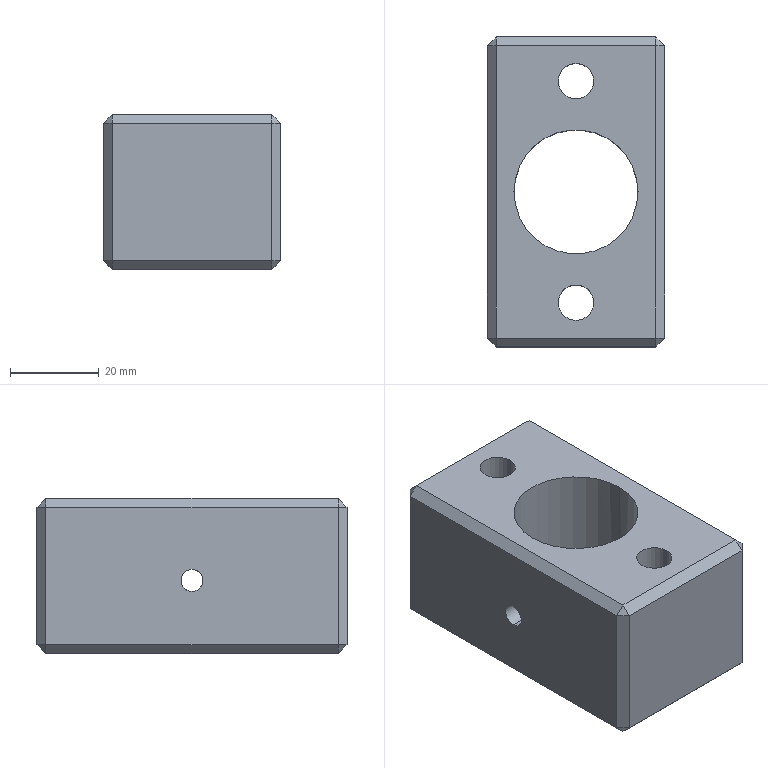Part | SolidWorks | features ICE 2, MirrorPattern 2, 3DProfileFeature 1, Chamfer 1, Extrusion 1, HoleWzd 1 | 1 solid | 36 faces | box 40 x 70 x 35 mm | volume 71575 mm3 | plane 26 | cylinder 10 | commonest cylinder face diameters 5 x4 8 x4 28 x2
STEP:
#1=CARTESIAN_POINT('',(14.,0.,13.999));
#2=VERTEX_POINT('',#1);
#3=CARTESIAN_POINT('',(14.,0.,18.999));
#4=VERTEX_POINT('',#3);
#5=CARTESIAN_POINT('',(14.,0.,13.999));
#6=CARTESIAN_POINT('',(14.,-0.1655,13.999));
#7=CARTESIAN_POINT('',(13.997,-0.3282,14.015));
#8=CARTESIAN_POINT('',(13.986,-0.6482,14.079));
#9=CARTESIAN_POINT('',(13.978,-0.8072,14.127));
#10=CARTESIAN_POINT('',(13.957,-1.11,14.253));
#11=CARTESIAN_POINT('',(13.944,-1.253,14.33));
#12=CARTESIAN_POINT('',(13.917,-1.525,14.511));
#13=CARTESIAN_POINT('',(13.903,-1.653,14.616));
#14=CARTESIAN_POINT('',(13.859,-1.998,14.962));
#15=CARTESIAN_POINT('',(13.829,-2.184,15.24));
#16=CARTESIAN_POINT('',(13.798,-2.372,15.691));
#17=CARTESIAN_POINT('',(13.789,-2.42,15.849));
#18=CARTESIAN_POINT('',(13.778,-2.484,16.172));
#19=CARTESIAN_POINT('',(13.775,-2.5,16.334));
#20=CARTESIAN_POINT('',(13.775,-2.5,16.661));
#21=CARTESIAN_POINT('',(13.778,-2.484,16.827));
#22=CARTESIAN_POINT('',(13.789,-2.42,17.148));
#23=CARTESIAN_POINT('',(13.798,-2.372,17.304));
#24=CARTESIAN_POINT('',(13.819,-2.247,17.607));
#25=CARTESIAN_POINT('',(13.831,-2.169,17.753));
#26=CARTESIAN_POINT('',(13.858,-1.988,18.024));
#27=CARTESIAN_POINT('',(13.873,-1.884,18.15));
#28=CARTESIAN_POINT('',(13.903,-1.651,18.383));
#29=CARTESIAN_POINT('',(13.917,-1.525,18.486));
#30=CARTESIAN_POINT('',(13.944,-1.255,18.667));
#31=CARTESIAN_POINT('',(13.957,-1.109,18.746));
#32=CARTESIAN_POINT('',(13.978,-0.8062,18.871));
#33=CARTESIAN_POINT('',(13.986,-0.6504,18.918));
#34=CARTESIAN_POINT('',(13.997,-0.3293,18.982));
#35=CARTESIAN_POINT('',(14.,-0.1633,18.999));
#36=CARTESIAN_POINT('',(14.,0.,18.999));
#37=B_SPLINE_CURVE_WITH_KNOTS('',3,(#5,#6,#7,#8,#9,#10,#11,#12,#13,#14,#15,#16,#17,#18,#19,#20,#21,#22,#23,#24,#25,#26,#27,#28,#29,#30,#31,#32,#33,#34,#35,#36),.UNSPECIFIED.,.F.,.F.,(4,2,2,2,2,2,2,2,2,2,2,2,2,2,2,4),(0.,0.0004895,0.000979,0.001468,0.001958,0.002937,0.003426,0.003916,0.004405,0.004895,0.005384,0.005874,0.006363,0.006853,0.007342,0.007832),.UNSPECIFIED.);
#38=EDGE_CURVE('',#2,#4,#37,.T.);
#39=ORIENTED_EDGE('',*,*,#38,.T.);
#40=CARTESIAN_POINT('',(20.,0.,18.999));
#41=VERTEX_POINT('',#40);
#42=CARTESIAN_POINT('',(20.,0.,18.999));
#43=DIRECTION('',(1.,0.,0.));
#44=VECTOR('',#43,1000.);
#45=LINE('',#42,#44);
#46=EDGE_CURVE('',#4,#41,#45,.T.);
#47=ORIENTED_EDGE('',*,*,#46,.T.);
#48=CARTESIAN_POINT('',(20.,0.,13.999));
#49=VERTEX_POINT('',#48);
#50=CARTESIAN_POINT('',(20.,0.,16.499));
#51=DIRECTION('',(1.,0.,0.));
#52=DIRECTION('',(0.,0.,-1.));
#53=AXIS2_PLACEMENT_3D('',#50,#51,#52);
#54=CIRCLE('',#53,2.5);
#55=EDGE_CURVE('',#41,#49,#54,.T.);
#56=ORIENTED_EDGE('',*,*,#55,.T.);
#57=CARTESIAN_POINT('',(20.,0.,13.999));
#58=DIRECTION('',(1.,0.,0.));
#59=VECTOR('',#58,1000.);
#60=LINE('',#57,#59);
#61=EDGE_CURVE('',#2,#49,#60,.T.);
#62=ORIENTED_EDGE('',*,*,#61,.F.);
#63=EDGE_LOOP('',(#39,#47,#56,#62));
#64=FACE_OUTER_BOUND('',#63,.T.);
#65=CARTESIAN_POINT('',(20.,0.,16.499));
#66=DIRECTION('',(1.,0.,0.));
#67=DIRECTION('',(0.,0.,-1.));
#68=AXIS2_PLACEMENT_3D('',#65,#66,#67);
#69=CYLINDRICAL_SURFACE('',#68,2.5);
#70=ADVANCED_FACE('',(#64),#69,.F.);
#71=CARTESIAN_POINT('',(-4.,-25.,0.));
#72=VERTEX_POINT('',#71);
#73=CARTESIAN_POINT('',(4.,-25.,0.));
#74=VERTEX_POINT('',#73);
#75=CARTESIAN_POINT('',(0.,-25.,0.));
#76=DIRECTION('',(0.,0.,1.));
#77=DIRECTION('',(-1.,0.,0.));
#78=AXIS2_PLACEMENT_3D('',#75,#76,#77);
#79=CIRCLE('',#78,4.);
#80=EDGE_CURVE('',#72,#74,#79,.T.);
#81=ORIENTED_EDGE('',*,*,#80,.F.);
#82=CARTESIAN_POINT('',(-4.,-25.,35.));
#83=VERTEX_POINT('',#82);
#84=CARTESIAN_POINT('',(-4.,-25.,-24.));
#85=DIRECTION('',(0.,0.,1.));
#86=VECTOR('',#85,1000.);
#87=LINE('',#84,#86);
#88=EDGE_CURVE('',#72,#83,#87,.T.);
#89=ORIENTED_EDGE('',*,*,#88,.T.);
#90=CARTESIAN_POINT('',(4.,-25.,35.));
#91=VERTEX_POINT('',#90);
#92=CARTESIAN_POINT('',(0.,-25.,35.));
#93=DIRECTION('',(0.,0.,-1.));
#94=DIRECTION('',(1.,0.,0.));
#95=AXIS2_PLACEMENT_3D('',#92,#93,#94);
#96=CIRCLE('',#95,4.);
#97=EDGE_CURVE('',#91,#83,#96,.T.);
#98=ORIENTED_EDGE('',*,*,#97,.F.);
#99=CARTESIAN_POINT('',(4.,-25.,-24.));
#100=DIRECTION('',(0.,0.,1.));
#101=VECTOR('',#100,1000.);
#102=LINE('',#99,#101);
#103=EDGE_CURVE('',#74,#91,#102,.T.);
#104=ORIENTED_EDGE('',*,*,#103,.F.);
#105=EDGE_LOOP('',(#81,#89,#98,#104));
#106=FACE_OUTER_BOUND('',#105,.T.);
#107=CARTESIAN_POINT('',(0.,-25.,-24.));
#108=DIRECTION('',(0.,0.,1.));
#109=DIRECTION('',(1.,0.,0.));
#110=AXIS2_PLACEMENT_3D('',#107,#108,#109);
#111=CYLINDRICAL_SURFACE('',#110,4.);
#112=ADVANCED_FACE('',(#106),#111,.F.);
#113=CARTESIAN_POINT('',(-14.,0.,13.999));
#114=VERTEX_POINT('',#113);
#115=CARTESIAN_POINT('',(-14.,0.,18.999));
#116=VERTEX_POINT('',#115);
#117=CARTESIAN_POINT('',(-14.,0.,13.999));
#118=CARTESIAN_POINT('',(-14.,-0.3266,13.999));
#119=CARTESIAN_POINT('',(-13.988,-0.6561,14.065));
#120=CARTESIAN_POINT('',(-13.957,-1.108,14.252));
#121=CARTESIAN_POINT('',(-13.944,-1.253,14.33));
#122=CARTESIAN_POINT('',(-13.917,-1.526,14.512));
#123=CARTESIAN_POINT('',(-13.903,-1.651,14.615));
#124=CARTESIAN_POINT('',(-13.873,-1.882,14.845));
#125=CARTESIAN_POINT('',(-13.859,-1.987,14.973));
#126=CARTESIAN_POINT('',(-13.831,-2.169,15.244));
#127=CARTESIAN_POINT('',(-13.819,-2.246,15.388));
#128=CARTESIAN_POINT('',(-13.798,-2.371,15.691));
#129=CARTESIAN_POINT('',(-13.789,-2.42,15.849));
#130=CARTESIAN_POINT('',(-13.778,-2.483,16.169));
#131=CARTESIAN_POINT('',(-13.775,-2.5,16.332));
#132=CARTESIAN_POINT('',(-13.775,-2.5,16.663));
#133=CARTESIAN_POINT('',(-13.778,-2.484,16.825));
#134=CARTESIAN_POINT('',(-13.789,-2.42,17.145));
#135=CARTESIAN_POINT('',(-13.798,-2.372,17.305));
#136=CARTESIAN_POINT('',(-13.819,-2.247,17.607));
#137=CARTESIAN_POINT('',(-13.831,-2.17,17.75));
#138=CARTESIAN_POINT('',(-13.858,-1.989,18.022));
#139=CARTESIAN_POINT('',(-13.873,-1.884,18.15));
#140=CARTESIAN_POINT('',(-13.917,-1.539,18.496));
#141=CARTESIAN_POINT('',(-13.946,-1.261,18.682));
#142=CARTESIAN_POINT('',(-13.977,-0.81,18.87));
#143=CARTESIAN_POINT('',(-13.986,-0.6517,18.918));
#144=CARTESIAN_POINT('',(-13.997,-0.3289,18.983));
#145=CARTESIAN_POINT('',(-14.,-0.1655,18.999));
#146=CARTESIAN_POINT('',(-14.,0.,18.999));
#147=B_SPLINE_CURVE_WITH_KNOTS('',3,(#117,#118,#119,#120,#121,#122,#123,#124,#125,#126,#127,#128,#129,#130,#131,#132,#133,#134,#135,#136,#137,#138,#139,#140,#141,#142,#143,#144,#145,#146),.UNSPECIFIED.,.F.,.F.,(4,2,2,2,2,2,2,2,2,2,2,2,2,2,4),(0.007832,0.008811,0.0093,0.009789,0.01028,0.01077,0.01126,0.01175,0.01224,0.01273,0.01321,0.0137,0.01468,0.01517,0.01566),.UNSPECIFIED.);
#148=EDGE_CURVE('',#114,#116,#147,.T.);
#149=ORIENTED_EDGE('',*,*,#148,.F.);
#150=CARTESIAN_POINT('',(-20.,0.,13.999));
#151=VERTEX_POINT('',#150);
#152=CARTESIAN_POINT('',(-20.,0.,13.999));
#153=DIRECTION('',(-1.,0.,0.));
#154=VECTOR('',#153,1000.);
#155=LINE('',#152,#154);
#156=EDGE_CURVE('',#114,#151,#155,.T.);
#157=ORIENTED_EDGE('',*,*,#156,.T.);
#158=CARTESIAN_POINT('',(-20.,0.,18.999));
#159=VERTEX_POINT('',#158);
#160=CARTESIAN_POINT('',(-20.,0.,16.499));
#161=DIRECTION('',(-1.,0.,0.));
#162=DIRECTION('',(0.,0.,1.));
#163=AXIS2_PLACEMENT_3D('',#160,#161,#162);
#164=CIRCLE('',#163,2.5);
#165=EDGE_CURVE('',#151,#159,#164,.T.);
#166=ORIENTED_EDGE('',*,*,#165,.T.);
#167=CARTESIAN_POINT('',(-20.,0.,18.999));
#168=DIRECTION('',(-1.,0.,0.));
#169=VECTOR('',#168,1000.);
#170=LINE('',#167,#169);
#171=EDGE_CURVE('',#116,#159,#170,.T.);
#172=ORIENTED_EDGE('',*,*,#171,.F.);
#173=EDGE_LOOP('',(#149,#157,#166,#172));
#174=FACE_OUTER_BOUND('',#173,.T.);
#175=CARTESIAN_POINT('',(-20.,0.,16.499));
#176=DIRECTION('',(-1.,0.,0.));
#177=DIRECTION('',(0.,0.,1.));
#178=AXIS2_PLACEMENT_3D('',#175,#176,#177);
#179=CYLINDRICAL_SURFACE('',#178,2.5);
#180=ADVANCED_FACE('',(#174),#179,.F.);
#181=CARTESIAN_POINT('',(4.,25.,0.));
#182=VERTEX_POINT('',#181);
#183=CARTESIAN_POINT('',(-4.,25.,0.));
#184=VERTEX_POINT('',#183);
#185=CARTESIAN_POINT('',(0.,25.,0.));
#186=DIRECTION('',(0.,0.,-1.));
#187=DIRECTION('',(-1.,0.,0.));
#188=AXIS2_PLACEMENT_3D('',#185,#186,#187);
#189=CIRCLE('',#188,4.);
#190=EDGE_CURVE('',#182,#184,#189,.T.);
#191=ORIENTED_EDGE('',*,*,#190,.T.);
#192=CARTESIAN_POINT('',(-4.,25.,35.));
#193=VERTEX_POINT('',#192);
#194=CARTESIAN_POINT('',(-4.,25.,-24.));
#195=DIRECTION('',(0.,0.,1.));
#196=VECTOR('',#195,1000.);
#197=LINE('',#194,#196);
#198=EDGE_CURVE('',#184,#193,#197,.T.);
#199=ORIENTED_EDGE('',*,*,#198,.T.);
#200=CARTESIAN_POINT('',(4.,25.,35.));
#201=VERTEX_POINT('',#200);
#202=CARTESIAN_POINT('',(0.,25.,35.));
#203=DIRECTION('',(0.,0.,1.));
#204=DIRECTION('',(1.,0.,0.));
#205=AXIS2_PLACEMENT_3D('',#202,#203,#204);
#206=CIRCLE('',#205,4.);
#207=EDGE_CURVE('',#193,#201,#206,.T.);
#208=ORIENTED_EDGE('',*,*,#207,.T.);
#209=CARTESIAN_POINT('',(4.,25.,-24.));
#210=DIRECTION('',(0.,0.,1.));
#211=VECTOR('',#210,1000.);
#212=LINE('',#209,#211);
#213=EDGE_CURVE('',#182,#201,#212,.T.);
#214=ORIENTED_EDGE('',*,*,#213,.F.);
#215=EDGE_LOOP('',(#191,#199,#208,#214));
#216=FACE_OUTER_BOUND('',#215,.T.);
#217=CARTESIAN_POINT('',(0.,25.,-24.));
#218=DIRECTION('',(0.,0.,1.));
#219=DIRECTION('',(1.,0.,0.));
#220=AXIS2_PLACEMENT_3D('',#217,#218,#219);
#221=CYLINDRICAL_SURFACE('',#220,4.);
#222=ADVANCED_FACE('',(#216),#221,.F.);
#223=CARTESIAN_POINT('',(14.,0.,0.));
#224=VERTEX_POINT('',#223);
#225=CARTESIAN_POINT('',(-14.,0.,0.));
#226=VERTEX_POINT('',#225);
#227=CARTESIAN_POINT('',(0.,0.,0.));
#228=DIRECTION('',(0.,0.,-1.));
#229=DIRECTION('',(-1.,0.,0.));
#230=AXIS2_PLACEMENT_3D('',#227,#228,#229);
#231=CIRCLE('',#230,14.);
#232=EDGE_CURVE('',#224,#226,#231,.T.);
#233=ORIENTED_EDGE('',*,*,#232,.T.);
#234=CARTESIAN_POINT('',(-14.,0.,-29.));
#235=DIRECTION('',(0.,0.,1.));
#236=VECTOR('',#235,1000.);
#237=LINE('',#234,#236);
#238=EDGE_CURVE('',#226,#114,#237,.T.);
#239=ORIENTED_EDGE('',*,*,#238,.T.);
#240=ORIENTED_EDGE('',*,*,#148,.T.);
#241=CARTESIAN_POINT('',(-14.,0.,35.));
#242=VERTEX_POINT('',#241);
#243=CARTESIAN_POINT('',(-14.,0.,-29.));
#244=DIRECTION('',(0.,0.,1.));
#245=VECTOR('',#244,1000.);
#246=LINE('',#243,#245);
#247=EDGE_CURVE('',#116,#242,#246,.T.);
#248=ORIENTED_EDGE('',*,*,#247,.T.);
#249=CARTESIAN_POINT('',(14.,0.,35.));
#250=VERTEX_POINT('',#249);
#251=CARTESIAN_POINT('',(0.,0.,35.));
#252=DIRECTION('',(0.,0.,1.));
#253=DIRECTION('',(1.,0.,0.));
#254=AXIS2_PLACEMENT_3D('',#251,#252,#253);
#255=CIRCLE('',#254,14.);
#256=EDGE_CURVE('',#242,#250,#255,.T.);
#257=ORIENTED_EDGE('',*,*,#256,.T.);
#258=CARTESIAN_POINT('',(14.,0.,-29.));
#259=DIRECTION('',(0.,0.,1.));
#260=VECTOR('',#259,1000.);
#261=LINE('',#258,#260);
#262=EDGE_CURVE('',#4,#250,#261,.T.);
#263=ORIENTED_EDGE('',*,*,#262,.F.);
#264=ORIENTED_EDGE('',*,*,#38,.F.);
#265=CARTESIAN_POINT('',(14.,0.,-29.));
#266=DIRECTION('',(0.,0.,1.));
#267=VECTOR('',#266,1000.);
#268=LINE('',#265,#267);
#269=EDGE_CURVE('',#224,#2,#268,.T.);
#270=ORIENTED_EDGE('',*,*,#269,.F.);
#271=EDGE_LOOP('',(#233,#239,#240,#248,#257,#263,#264,#270));
#272=FACE_OUTER_BOUND('',#271,.T.);
#273=CARTESIAN_POINT('',(0.,0.,-29.));
#274=DIRECTION('',(0.,0.,1.));
#275=DIRECTION('',(1.,0.,0.));
#276=AXIS2_PLACEMENT_3D('',#273,#274,#275);
#277=CYLINDRICAL_SURFACE('',#276,14.);
#278=ADVANCED_FACE('',(#272),#277,.F.);
#279=CARTESIAN_POINT('',(-20.,-33.,2.));
#280=VERTEX_POINT('',#279);
#281=CARTESIAN_POINT('',(-20.,-33.,33.));
#282=VERTEX_POINT('',#281);
#283=CARTESIAN_POINT('',(-20.,-33.,35.));
#284=DIRECTION('',(0.,0.,1.));
#285=VECTOR('',#284,1000.);
#286=LINE('',#283,#285);
#287=EDGE_CURVE('',#280,#282,#286,.T.);
#288=ORIENTED_EDGE('',*,*,#287,.T.);
#289=CARTESIAN_POINT('',(-20.,33.,33.));
#290=VERTEX_POINT('',#289);
#291=CARTESIAN_POINT('',(-20.,-35.,33.));
#292=DIRECTION('',(0.,1.,0.));
#293=VECTOR('',#292,1000.);
#294=LINE('',#291,#293);
#295=EDGE_CURVE('',#282,#290,#294,.T.);
#296=ORIENTED_EDGE('',*,*,#295,.T.);
#297=CARTESIAN_POINT('',(-20.,33.,2.));
#298=VERTEX_POINT('',#297);
#299=CARTESIAN_POINT('',(-20.,33.,35.));
#300=DIRECTION('',(0.,0.,-1.));
#301=VECTOR('',#300,1000.);
#302=LINE('',#299,#301);
#303=EDGE_CURVE('',#290,#298,#302,.T.);
#304=ORIENTED_EDGE('',*,*,#303,.T.);
#305=CARTESIAN_POINT('',(-20.,-35.,2.));
#306=DIRECTION('',(0.,-1.,0.));
#307=VECTOR('',#306,1000.);
#308=LINE('',#305,#307);
#309=EDGE_CURVE('',#298,#280,#308,.T.);
#310=ORIENTED_EDGE('',*,*,#309,.T.);
#311=EDGE_LOOP('',(#288,#296,#304,#310));
#312=FACE_OUTER_BOUND('',#311,.T.);
#313=CARTESIAN_POINT('',(-20.,0.,16.499));
#314=DIRECTION('',(-1.,0.,0.));
#315=DIRECTION('',(0.,0.,1.));
#316=AXIS2_PLACEMENT_3D('',#313,#314,#315);
#317=CIRCLE('',#316,2.5);
#318=EDGE_CURVE('',#159,#151,#317,.T.);
#319=ORIENTED_EDGE('',*,*,#318,.F.);
#320=ORIENTED_EDGE('',*,*,#165,.F.);
#321=EDGE_LOOP('',(#319,#320));
#322=FACE_BOUND('',#321,.T.);
#323=CARTESIAN_POINT('',(-20.,-35.,35.));
#324=DIRECTION('',(1.,0.,0.));
#325=DIRECTION('',(0.,0.,-1.));
#326=AXIS2_PLACEMENT_3D('',#323,#324,#325);
#327=PLANE('',#326);
#328=ADVANCED_FACE('',(#312,#322),#327,.F.);
#329=CARTESIAN_POINT('',(20.,33.,33.));
#330=VERTEX_POINT('',#329);
#331=CARTESIAN_POINT('',(20.,-33.,33.));
#332=VERTEX_POINT('',#331);
#333=CARTESIAN_POINT('',(20.,-35.,33.));
#334=DIRECTION('',(0.,-1.,0.));
#335=VECTOR('',#334,1000.);
#336=LINE('',#333,#335);
#337=EDGE_CURVE('',#330,#332,#336,.T.);
#338=ORIENTED_EDGE('',*,*,#337,.T.);
#339=CARTESIAN_POINT('',(20.,-33.,2.));
#340=VERTEX_POINT('',#339);
#341=CARTESIAN_POINT('',(20.,-33.,35.));
#342=DIRECTION('',(0.,0.,-1.));
#343=VECTOR('',#342,1000.);
#344=LINE('',#341,#343);
#345=EDGE_CURVE('',#332,#340,#344,.T.);
#346=ORIENTED_EDGE('',*,*,#345,.T.);
#347=CARTESIAN_POINT('',(20.,33.,2.));
#348=VERTEX_POINT('',#347);
#349=CARTESIAN_POINT('',(20.,35.,2.));
#350=DIRECTION('',(0.,1.,0.));
#351=VECTOR('',#350,1000.);
#352=LINE('',#349,#351);
#353=EDGE_CURVE('',#340,#348,#352,.T.);
#354=ORIENTED_EDGE('',*,*,#353,.T.);
#355=CARTESIAN_POINT('',(20.,33.,35.));
#356=DIRECTION('',(0.,0.,1.));
#357=VECTOR('',#356,1000.);
#358=LINE('',#355,#357);
#359=EDGE_CURVE('',#348,#330,#358,.T.);
#360=ORIENTED_EDGE('',*,*,#359,.T.);
#361=EDGE_LOOP('',(#338,#346,#354,#360));
#362=FACE_OUTER_BOUND('',#361,.T.);
#363=CARTESIAN_POINT('',(20.,0.,16.499));
#364=DIRECTION('',(1.,0.,0.));
#365=DIRECTION('',(0.,0.,-1.));
#366=AXIS2_PLACEMENT_3D('',#363,#364,#365);
#367=CIRCLE('',#366,2.5);
#368=EDGE_CURVE('',#49,#41,#367,.T.);
#369=ORIENTED_EDGE('',*,*,#368,.F.);
#370=ORIENTED_EDGE('',*,*,#55,.F.);
#371=EDGE_LOOP('',(#369,#370));
#372=FACE_BOUND('',#371,.T.);
#373=CARTESIAN_POINT('',(20.,-35.,35.));
#374=DIRECTION('',(-1.,0.,0.));
#375=DIRECTION('',(0.,0.,1.));
#376=AXIS2_PLACEMENT_3D('',#373,#374,#375);
#377=PLANE('',#376);
#378=ADVANCED_FACE('',(#362,#372),#377,.F.);
#379=CARTESIAN_POINT('',(18.,35.,2.));
#380=VERTEX_POINT('',#379);
#381=CARTESIAN_POINT('',(-18.,35.,2.));
#382=VERTEX_POINT('',#381);
#383=CARTESIAN_POINT('',(-20.,35.,2.));
#384=DIRECTION('',(-1.,0.,0.));
#385=VECTOR('',#384,1000.);
#386=LINE('',#383,#385);
#387=EDGE_CURVE('',#380,#382,#386,.T.);
#388=ORIENTED_EDGE('',*,*,#387,.T.);
#389=CARTESIAN_POINT('',(-18.,35.,33.));
#390=VERTEX_POINT('',#389);
#391=CARTESIAN_POINT('',(-18.,35.,35.));
#392=DIRECTION('',(0.,0.,1.));
#393=VECTOR('',#392,1000.);
#394=LINE('',#391,#393);
#395=EDGE_CURVE('',#382,#390,#394,.T.);
#396=ORIENTED_EDGE('',*,*,#395,.T.);
#397=CARTESIAN_POINT('',(18.,35.,33.));
#398=VERTEX_POINT('',#397);
#399=CARTESIAN_POINT('',(-20.,35.,33.));
#400=DIRECTION('',(1.,0.,0.));
#401=VECTOR('',#400,1000.);
#402=LINE('',#399,#401);
#403=EDGE_CURVE('',#390,#398,#402,.T.);
#404=ORIENTED_EDGE('',*,*,#403,.T.);
#405=CARTESIAN_POINT('',(18.,35.,35.));
#406=DIRECTION('',(0.,0.,-1.));
#407=VECTOR('',#406,1000.);
#408=LINE('',#405,#407);
#409=EDGE_CURVE('',#398,#380,#408,.T.);
#410=ORIENTED_EDGE('',*,*,#409,.T.);
#411=EDGE_LOOP('',(#388,#396,#404,#410));
#412=FACE_OUTER_BOUND('',#411,.T.);
#413=CARTESIAN_POINT('',(-20.,35.,35.));
#414=DIRECTION('',(0.,-1.,0.));
#415=DIRECTION('',(0.,0.,-1.));
#416=AXIS2_PLACEMENT_3D('',#413,#414,#415);
#417=PLANE('',#416);
#418=ADVANCED_FACE('',(#412),#417,.F.);
#419=CARTESIAN_POINT('',(18.,-35.,33.));
#420=VERTEX_POINT('',#419);
#421=CARTESIAN_POINT('',(-18.,-35.,33.));
#422=VERTEX_POINT('',#421);
#423=CARTESIAN_POINT('',(-20.,-35.,33.));
#424=DIRECTION('',(-1.,0.,0.));
#425=VECTOR('',#424,1000.);
#426=LINE('',#423,#425);
#427=EDGE_CURVE('',#420,#422,#426,.T.);
#428=ORIENTED_EDGE('',*,*,#427,.T.);
#429=CARTESIAN_POINT('',(-18.,-35.,2.));
#430=VERTEX_POINT('',#429);
#431=CARTESIAN_POINT('',(-18.,-35.,35.));
#432=DIRECTION('',(0.,0.,-1.));
#433=VECTOR('',#432,1000.);
#434=LINE('',#431,#433);
#435=EDGE_CURVE('',#422,#430,#434,.T.);
#436=ORIENTED_EDGE('',*,*,#435,.T.);
#437=CARTESIAN_POINT('',(18.,-35.,2.));
#438=VERTEX_POINT('',#437);
#439=CARTESIAN_POINT('',(20.,-35.,2.));
#440=DIRECTION('',(1.,0.,0.));
#441=VECTOR('',#440,1000.);
#442=LINE('',#439,#441);
#443=EDGE_CURVE('',#430,#438,#442,.T.);
#444=ORIENTED_EDGE('',*,*,#443,.T.);
#445=CARTESIAN_POINT('',(18.,-35.,35.));
#446=DIRECTION('',(0.,0.,1.));
#447=VECTOR('',#446,1000.);
#448=LINE('',#445,#447);
#449=EDGE_CURVE('',#438,#420,#448,.T.);
#450=ORIENTED_EDGE('',*,*,#449,.T.);
#451=EDGE_LOOP('',(#428,#436,#444,#450));
#452=FACE_OUTER_BOUND('',#451,.T.);
#453=CARTESIAN_POINT('',(-20.,-35.,35.));
#454=DIRECTION('',(0.,1.,0.));
#455=DIRECTION('',(0.,0.,1.));
#456=AXIS2_PLACEMENT_3D('',#453,#454,#455);
#457=PLANE('',#456);
#458=ADVANCED_FACE('',(#452),#457,.F.);
#459=CARTESIAN_POINT('',(-18.,33.,35.));
#460=VERTEX_POINT('',#459);
#461=CARTESIAN_POINT('',(-18.,-33.,35.));
#462=VERTEX_POINT('',#461);
#463=CARTESIAN_POINT('',(-18.,0.,35.));
#464=DIRECTION('',(0.,-1.,0.));
#465=VECTOR('',#464,1000.);
#466=LINE('',#463,#465);
#467=EDGE_CURVE('',#460,#462,#466,.T.);
#468=ORIENTED_EDGE('',*,*,#467,.T.);
#469=CARTESIAN_POINT('',(18.,-33.,35.));
#470=VERTEX_POINT('',#469);
#471=CARTESIAN_POINT('',(0.,-33.,35.));
#472=DIRECTION('',(1.,0.,0.));
#473=VECTOR('',#472,1000.);
#474=LINE('',#471,#473);
#475=EDGE_CURVE('',#462,#470,#474,.T.);
#476=ORIENTED_EDGE('',*,*,#475,.T.);
#477=CARTESIAN_POINT('',(18.,33.,35.));
#478=VERTEX_POINT('',#477);
#479=CARTESIAN_POINT('',(18.,0.,35.));
#480=DIRECTION('',(0.,1.,0.));
#481=VECTOR('',#480,1000.);
#482=LINE('',#479,#481);
#483=EDGE_CURVE('',#470,#478,#482,.T.);
#484=ORIENTED_EDGE('',*,*,#483,.T.);
#485=CARTESIAN_POINT('',(0.,33.,35.));
#486=DIRECTION('',(-1.,0.,0.));
#487=VECTOR('',#486,1000.);
#488=LINE('',#485,#487);
#489=EDGE_CURVE('',#478,#460,#488,.T.);
#490=ORIENTED_EDGE('',*,*,#489,.T.);
#491=EDGE_LOOP('',(#468,#476,#484,#490));
#492=FACE_OUTER_BOUND('',#491,.T.);
#493=ORIENTED_EDGE('',*,*,#97,.T.);
#494=CARTESIAN_POINT('',(0.,-25.,35.));
#495=DIRECTION('',(0.,0.,-1.));
#496=DIRECTION('',(1.,0.,0.));
#497=AXIS2_PLACEMENT_3D('',#494,#495,#496);
#498=CIRCLE('',#497,4.);
#499=EDGE_CURVE('',#83,#91,#498,.T.);
#500=ORIENTED_EDGE('',*,*,#499,.T.);
#501=EDGE_LOOP('',(#493,#500));
#502=FACE_BOUND('',#501,.T.);
#503=CARTESIAN_POINT('',(0.,25.,35.));
#504=DIRECTION('',(0.,0.,1.));
#505=DIRECTION('',(1.,0.,0.));
#506=AXIS2_PLACEMENT_3D('',#503,#504,#505);
#507=CIRCLE('',#506,4.);
#508=EDGE_CURVE('',#201,#193,#507,.T.);
#509=ORIENTED_EDGE('',*,*,#508,.F.);
#510=ORIENTED_EDGE('',*,*,#207,.F.);
#511=EDGE_LOOP('',(#509,#510));
#512=FACE_BOUND('',#511,.T.);
#513=CARTESIAN_POINT('',(0.,0.,35.));
#514=DIRECTION('',(0.,0.,1.));
#515=DIRECTION('',(1.,0.,0.));
#516=AXIS2_PLACEMENT_3D('',#513,#514,#515);
#517=CIRCLE('',#516,14.);
#518=EDGE_CURVE('',#250,#242,#517,.T.);
#519=ORIENTED_EDGE('',*,*,#518,.F.);
#520=ORIENTED_EDGE('',*,*,#256,.F.);
#521=EDGE_LOOP('',(#519,#520));
#522=FACE_BOUND('',#521,.T.);
#523=CARTESIAN_POINT('',(0.,0.,35.));
#524=DIRECTION('',(0.,0.,-1.));
#525=DIRECTION('',(-1.,0.,0.));
#526=AXIS2_PLACEMENT_3D('',#523,#524,#525);
#527=PLANE('',#526);
#528=ADVANCED_FACE('',(#492,#502,#512,#522),#527,.F.);
#529=CARTESIAN_POINT('',(18.,33.,0.));
#530=VERTEX_POINT('',#529);
#531=CARTESIAN_POINT('',(18.,-33.,0.));
#532=VERTEX_POINT('',#531);
#533=CARTESIAN_POINT('',(18.,-35.,0.));
#534=DIRECTION('',(0.,-1.,0.));
#535=VECTOR('',#534,1000.);
#536=LINE('',#533,#535);
#537=EDGE_CURVE('',#530,#532,#536,.T.);
#538=ORIENTED_EDGE('',*,*,#537,.T.);
#539=CARTESIAN_POINT('',(-18.,-33.,0.));
#540=VERTEX_POINT('',#539);
#541=CARTESIAN_POINT('',(-20.,-33.,0.));
#542=DIRECTION('',(-1.,0.,0.));
#543=VECTOR('',#542,1000.);
#544=LINE('',#541,#543);
#545=EDGE_CURVE('',#532,#540,#544,.T.);
#546=ORIENTED_EDGE('',*,*,#545,.T.);
#547=CARTESIAN_POINT('',(-18.,33.,0.));
#548=VERTEX_POINT('',#547);
#549=CARTESIAN_POINT('',(-18.,35.,0.));
#550=DIRECTION('',(0.,1.,0.));
#551=VECTOR('',#550,1000.);
#552=LINE('',#549,#551);
#553=EDGE_CURVE('',#540,#548,#552,.T.);
#554=ORIENTED_EDGE('',*,*,#553,.T.);
#555=CARTESIAN_POINT('',(20.,33.,0.));
#556=DIRECTION('',(1.,0.,0.));
#557=VECTOR('',#556,1000.);
#558=LINE('',#555,#557);
#559=EDGE_CURVE('',#548,#530,#558,.T.);
#560=ORIENTED_EDGE('',*,*,#559,.T.);
#561=EDGE_LOOP('',(#538,#546,#554,#560));
#562=FACE_OUTER_BOUND('',#561,.T.);
#563=CARTESIAN_POINT('',(0.,-25.,0.));
#564=DIRECTION('',(0.,0.,1.));
#565=DIRECTION('',(-1.,0.,0.));
#566=AXIS2_PLACEMENT_3D('',#563,#564,#565);
#567=CIRCLE('',#566,4.);
#568=EDGE_CURVE('',#74,#72,#567,.T.);
#569=ORIENTED_EDGE('',*,*,#568,.T.);
#570=ORIENTED_EDGE('',*,*,#80,.T.);
#571=EDGE_LOOP('',(#569,#570));
#572=FACE_BOUND('',#571,.T.);
#573=ORIENTED_EDGE('',*,*,#190,.F.);
#574=CARTESIAN_POINT('',(0.,25.,0.));
#575=DIRECTION('',(0.,0.,-1.));
#576=DIRECTION('',(-1.,0.,0.));
#577=AXIS2_PLACEMENT_3D('',#574,#575,#576);
#578=CIRCLE('',#577,4.);
#579=EDGE_CURVE('',#184,#182,#578,.T.);
#580=ORIENTED_EDGE('',*,*,#579,.F.);
#581=EDGE_LOOP('',(#573,#580));
#582=FACE_BOUND('',#581,.T.);
#583=ORIENTED_EDGE('',*,*,#232,.F.);
#584=CARTESIAN_POINT('',(0.,0.,0.));
#585=DIRECTION('',(0.,0.,-1.));
#586=DIRECTION('',(-1.,0.,0.));
#587=AXIS2_PLACEMENT_3D('',#584,#585,#586);
#588=CIRCLE('',#587,14.);
#589=EDGE_CURVE('',#226,#224,#588,.T.);
#590=ORIENTED_EDGE('',*,*,#589,.F.);
#591=EDGE_LOOP('',(#583,#590));
#592=FACE_BOUND('',#591,.T.);
#593=CARTESIAN_POINT('',(0.,0.,0.));
#594=DIRECTION('',(0.,0.,-1.));
#595=DIRECTION('',(-1.,0.,0.));
#596=AXIS2_PLACEMENT_3D('',#593,#594,#595);
#597=PLANE('',#596);
#598=ADVANCED_FACE('',(#562,#572,#582,#592),#597,.T.);
#599=ORIENTED_EDGE('',*,*,#238,.F.);
#600=ORIENTED_EDGE('',*,*,#589,.T.);
#601=ORIENTED_EDGE('',*,*,#269,.T.);
#602=CARTESIAN_POINT('',(14.,0.,18.999));
#603=CARTESIAN_POINT('',(14.,0.3266,18.999));
#604=CARTESIAN_POINT('',(13.988,0.6561,18.933));
#605=CARTESIAN_POINT('',(13.957,1.108,18.746));
#606=CARTESIAN_POINT('',(13.944,1.253,18.668));
#607=CARTESIAN_POINT('',(13.917,1.526,18.486));
#608=CARTESIAN_POINT('',(13.903,1.651,18.383));
#609=CARTESIAN_POINT('',(13.873,1.882,18.153));
#610=CARTESIAN_POINT('',(13.859,1.987,18.024));
#611=CARTESIAN_POINT('',(13.831,2.169,17.753));
#612=CARTESIAN_POINT('',(13.819,2.246,17.61));
#613=CARTESIAN_POINT('',(13.798,2.371,17.307));
#614=CARTESIAN_POINT('',(13.789,2.42,17.149));
#615=CARTESIAN_POINT('',(13.778,2.483,16.829));
#616=CARTESIAN_POINT('',(13.775,2.5,16.665));
#617=CARTESIAN_POINT('',(13.775,2.5,16.335));
#618=CARTESIAN_POINT('',(13.778,2.484,16.173));
#619=CARTESIAN_POINT('',(13.789,2.42,15.852));
#620=CARTESIAN_POINT('',(13.798,2.372,15.693));
#621=CARTESIAN_POINT('',(13.819,2.247,15.391));
#622=CARTESIAN_POINT('',(13.831,2.17,15.247));
#623=CARTESIAN_POINT('',(13.858,1.989,14.975));
#624=CARTESIAN_POINT('',(13.873,1.884,14.847));
#625=CARTESIAN_POINT('',(13.917,1.539,14.502));
#626=CARTESIAN_POINT('',(13.946,1.261,14.316));
#627=CARTESIAN_POINT('',(13.977,0.81,14.128));
#628=CARTESIAN_POINT('',(13.986,0.6517,14.08));
#629=CARTESIAN_POINT('',(13.997,0.3289,14.015));
#630=CARTESIAN_POINT('',(14.,0.1655,13.999));
#631=CARTESIAN_POINT('',(14.,0.,13.999));
#632=B_SPLINE_CURVE_WITH_KNOTS('',3,(#602,#603,#604,#605,#606,#607,#608,#609,#610,#611,#612,#613,#614,#615,#616,#617,#618,#619,#620,#621,#622,#623,#624,#625,#626,#627,#628,#629,#630,#631),.UNSPECIFIED.,.F.,.F.,(4,2,2,2,2,2,2,2,2,2,2,2,2,2,4),(0.007832,0.008811,0.0093,0.009789,0.01028,0.01077,0.01126,0.01175,0.01224,0.01273,0.01321,0.0137,0.01468,0.01517,0.01566),.UNSPECIFIED.);
#633=EDGE_CURVE('',#4,#2,#632,.T.);
#634=ORIENTED_EDGE('',*,*,#633,.F.);
#635=ORIENTED_EDGE('',*,*,#262,.T.);
#636=ORIENTED_EDGE('',*,*,#518,.T.);
#637=ORIENTED_EDGE('',*,*,#247,.F.);
#638=CARTESIAN_POINT('',(-14.,0.,18.999));
#639=CARTESIAN_POINT('',(-14.,0.1655,18.999));
#640=CARTESIAN_POINT('',(-13.997,0.3282,18.983));
#641=CARTESIAN_POINT('',(-13.986,0.6482,18.919));
#642=CARTESIAN_POINT('',(-13.978,0.8072,18.871));
#643=CARTESIAN_POINT('',(-13.957,1.11,18.745));
#644=CARTESIAN_POINT('',(-13.944,1.253,18.668));
#645=CARTESIAN_POINT('',(-13.917,1.525,18.487));
#646=CARTESIAN_POINT('',(-13.903,1.653,18.381));
#647=CARTESIAN_POINT('',(-13.859,1.998,18.036));
#648=CARTESIAN_POINT('',(-13.829,2.184,17.758));
#649=CARTESIAN_POINT('',(-13.798,2.372,17.306));
#650=CARTESIAN_POINT('',(-13.789,2.42,17.149));
#651=CARTESIAN_POINT('',(-13.778,2.484,16.826));
#652=CARTESIAN_POINT('',(-13.775,2.5,16.663));
#653=CARTESIAN_POINT('',(-13.775,2.5,16.336));
#654=CARTESIAN_POINT('',(-13.778,2.484,16.17));
#655=CARTESIAN_POINT('',(-13.789,2.42,15.849));
#656=CARTESIAN_POINT('',(-13.798,2.372,15.693));
#657=CARTESIAN_POINT('',(-13.819,2.247,15.39));
#658=CARTESIAN_POINT('',(-13.831,2.169,15.244));
#659=CARTESIAN_POINT('',(-13.858,1.988,14.974));
#660=CARTESIAN_POINT('',(-13.873,1.884,14.847));
#661=CARTESIAN_POINT('',(-13.903,1.651,14.615));
#662=CARTESIAN_POINT('',(-13.917,1.525,14.512));
#663=CARTESIAN_POINT('',(-13.944,1.255,14.331));
#664=CARTESIAN_POINT('',(-13.957,1.109,14.252));
#665=CARTESIAN_POINT('',(-13.978,0.8062,14.127));
#666=CARTESIAN_POINT('',(-13.986,0.6504,14.079));
#667=CARTESIAN_POINT('',(-13.997,0.3293,14.015));
#668=CARTESIAN_POINT('',(-14.,0.1633,13.999));
#669=CARTESIAN_POINT('',(-14.,0.,13.999));
#670=B_SPLINE_CURVE_WITH_KNOTS('',3,(#638,#639,#640,#641,#642,#643,#644,#645,#646,#647,#648,#649,#650,#651,#652,#653,#654,#655,#656,#657,#658,#659,#660,#661,#662,#663,#664,#665,#666,#667,#668,#669),.UNSPECIFIED.,.F.,.F.,(4,2,2,2,2,2,2,2,2,2,2,2,2,2,2,4),(0.,0.0004895,0.000979,0.001468,0.001958,0.002937,0.003426,0.003916,0.004405,0.004895,0.005384,0.005874,0.006363,0.006853,0.007342,0.007832),.UNSPECIFIED.);
#671=EDGE_CURVE('',#116,#114,#670,.T.);
#672=ORIENTED_EDGE('',*,*,#671,.T.);
#673=EDGE_LOOP('',(#599,#600,#601,#634,#635,#636,#637,#672));
#674=FACE_OUTER_BOUND('',#673,.T.);
#675=CARTESIAN_POINT('',(0.,0.,-29.));
#676=DIRECTION('',(0.,0.,1.));
#677=DIRECTION('',(1.,0.,0.));
#678=AXIS2_PLACEMENT_3D('',#675,#676,#677);
#679=CYLINDRICAL_SURFACE('',#678,14.);
#680=ADVANCED_FACE('',(#674),#679,.F.);
#681=ORIENTED_EDGE('',*,*,#198,.F.);
#682=ORIENTED_EDGE('',*,*,#579,.T.);
#683=ORIENTED_EDGE('',*,*,#213,.T.);
#684=ORIENTED_EDGE('',*,*,#508,.T.);
#685=EDGE_LOOP('',(#681,#682,#683,#684));
#686=FACE_OUTER_BOUND('',#685,.T.);
#687=CARTESIAN_POINT('',(0.,25.,-24.));
#688=DIRECTION('',(0.,0.,1.));
#689=DIRECTION('',(1.,0.,0.));
#690=AXIS2_PLACEMENT_3D('',#687,#688,#689);
#691=CYLINDRICAL_SURFACE('',#690,4.);
#692=ADVANCED_FACE('',(#686),#691,.F.);
#693=ORIENTED_EDGE('',*,*,#156,.F.);
#694=ORIENTED_EDGE('',*,*,#671,.F.);
#695=ORIENTED_EDGE('',*,*,#171,.T.);
#696=ORIENTED_EDGE('',*,*,#318,.T.);
#697=EDGE_LOOP('',(#693,#694,#695,#696));
#698=FACE_OUTER_BOUND('',#697,.T.);
#699=CARTESIAN_POINT('',(-20.,0.,16.499));
#700=DIRECTION('',(-1.,0.,0.));
#701=DIRECTION('',(0.,0.,1.));
#702=AXIS2_PLACEMENT_3D('',#699,#700,#701);
#703=CYLINDRICAL_SURFACE('',#702,2.5);
#704=ADVANCED_FACE('',(#698),#703,.F.);
#705=ORIENTED_EDGE('',*,*,#88,.F.);
#706=ORIENTED_EDGE('',*,*,#568,.F.);
#707=ORIENTED_EDGE('',*,*,#103,.T.);
#708=ORIENTED_EDGE('',*,*,#499,.F.);
#709=EDGE_LOOP('',(#705,#706,#707,#708));
#710=FACE_OUTER_BOUND('',#709,.T.);
#711=CARTESIAN_POINT('',(0.,-25.,-24.));
#712=DIRECTION('',(0.,0.,1.));
#713=DIRECTION('',(1.,0.,0.));
#714=AXIS2_PLACEMENT_3D('',#711,#712,#713);
#715=CYLINDRICAL_SURFACE('',#714,4.);
#716=ADVANCED_FACE('',(#710),#715,.F.);
#717=ORIENTED_EDGE('',*,*,#46,.F.);
#718=ORIENTED_EDGE('',*,*,#633,.T.);
#719=ORIENTED_EDGE('',*,*,#61,.T.);
#720=ORIENTED_EDGE('',*,*,#368,.T.);
#721=EDGE_LOOP('',(#717,#718,#719,#720));
#722=FACE_OUTER_BOUND('',#721,.T.);
#723=CARTESIAN_POINT('',(20.,0.,16.499));
#724=DIRECTION('',(1.,0.,0.));
#725=DIRECTION('',(0.,0.,-1.));
#726=AXIS2_PLACEMENT_3D('',#723,#724,#725);
#727=CYLINDRICAL_SURFACE('',#726,2.5);
#728=ADVANCED_FACE('',(#722),#727,.F.);
#729=CARTESIAN_POINT('',(18.,35.,33.));
#730=DIRECTION('',(-0.7071,0.7071,0.));
#731=VECTOR('',#730,1000.);
#732=LINE('',#729,#731);
#733=EDGE_CURVE('',#330,#398,#732,.T.);
#734=ORIENTED_EDGE('',*,*,#733,.F.);
#735=ORIENTED_EDGE('',*,*,#359,.F.);
#736=CARTESIAN_POINT('',(19.,34.,2.));
#737=DIRECTION('',(0.7071,-0.7071,0.));
#738=VECTOR('',#737,1000.);
#739=LINE('',#736,#738);
#740=EDGE_CURVE('',#380,#348,#739,.T.);
#741=ORIENTED_EDGE('',*,*,#740,.F.);
#742=ORIENTED_EDGE('',*,*,#409,.F.);
#743=EDGE_LOOP('',(#734,#735,#741,#742));
#744=FACE_OUTER_BOUND('',#743,.T.);
#745=CARTESIAN_POINT('',(18.,35.,35.));
#746=DIRECTION('',(-0.7071,-0.7071,0.));
#747=DIRECTION('',(0.,0.,-1.));
#748=AXIS2_PLACEMENT_3D('',#745,#746,#747);
#749=PLANE('',#748);
#750=ADVANCED_FACE('',(#744),#749,.F.);
#751=CARTESIAN_POINT('',(19.,33.,34.));
#752=DIRECTION('',(-0.7071,0.,0.7071));
#753=VECTOR('',#752,1000.);
#754=LINE('',#751,#753);
#755=EDGE_CURVE('',#330,#478,#754,.T.);
#756=ORIENTED_EDGE('',*,*,#755,.F.);
#757=ORIENTED_EDGE('',*,*,#733,.T.);
#758=CARTESIAN_POINT('',(18.,35.,33.));
#759=DIRECTION('',(0.,0.7071,-0.7071));
#760=VECTOR('',#759,1000.);
#761=LINE('',#758,#760);
#762=EDGE_CURVE('',#478,#398,#761,.T.);
#763=ORIENTED_EDGE('',*,*,#762,.F.);
#764=EDGE_LOOP('',(#756,#757,#763));
#765=FACE_OUTER_BOUND('',#764,.T.);
#766=CARTESIAN_POINT('',(18.,35.,33.));
#767=DIRECTION('',(0.5774,0.5774,0.5774));
#768=DIRECTION('',(0.7071,0.,-0.7071));
#769=AXIS2_PLACEMENT_3D('',#766,#767,#768);
#770=PLANE('',#769);
#771=ADVANCED_FACE('',(#765),#770,.T.);
#772=CARTESIAN_POINT('',(18.,33.,0.));
#773=DIRECTION('',(0.,-0.7071,-0.7071));
#774=VECTOR('',#773,1000.);
#775=LINE('',#772,#774);
#776=EDGE_CURVE('',#380,#530,#775,.T.);
#777=ORIENTED_EDGE('',*,*,#776,.F.);
#778=ORIENTED_EDGE('',*,*,#740,.T.);
#779=CARTESIAN_POINT('',(18.,33.,0.));
#780=DIRECTION('',(0.7071,0.,0.7071));
#781=VECTOR('',#780,1000.);
#782=LINE('',#779,#781);
#783=EDGE_CURVE('',#530,#348,#782,.T.);
#784=ORIENTED_EDGE('',*,*,#783,.F.);
#785=EDGE_LOOP('',(#777,#778,#784));
#786=FACE_OUTER_BOUND('',#785,.T.);
#787=CARTESIAN_POINT('',(18.,33.,0.));
#788=DIRECTION('',(0.5774,0.5774,-0.5774));
#789=DIRECTION('',(-0.7071,0.,-0.7071));
#790=AXIS2_PLACEMENT_3D('',#787,#788,#789);
#791=PLANE('',#790);
#792=ADVANCED_FACE('',(#786),#791,.T.);
#793=ORIENTED_EDGE('',*,*,#762,.T.);
#794=ORIENTED_EDGE('',*,*,#403,.F.);
#795=CARTESIAN_POINT('',(-18.,35.,33.));
#796=DIRECTION('',(0.,0.7071,-0.7071));
#797=VECTOR('',#796,1000.);
#798=LINE('',#795,#797);
#799=EDGE_CURVE('',#460,#390,#798,.T.);
#800=ORIENTED_EDGE('',*,*,#799,.F.);
#801=ORIENTED_EDGE('',*,*,#489,.F.);
#802=EDGE_LOOP('',(#793,#794,#800,#801));
#803=FACE_OUTER_BOUND('',#802,.T.);
#804=CARTESIAN_POINT('',(0.,33.,35.));
#805=DIRECTION('',(0.,-0.7071,-0.7071));
#806=DIRECTION('',(-1.,0.,0.));
#807=AXIS2_PLACEMENT_3D('',#804,#805,#806);
#808=PLANE('',#807);
#809=ADVANCED_FACE('',(#803),#808,.F.);
#810=ORIENTED_EDGE('',*,*,#755,.T.);
#811=ORIENTED_EDGE('',*,*,#483,.F.);
#812=CARTESIAN_POINT('',(18.,-33.,35.));
#813=DIRECTION('',(-0.7071,0.,0.7071));
#814=VECTOR('',#813,1000.);
#815=LINE('',#812,#814);
#816=EDGE_CURVE('',#332,#470,#815,.T.);
#817=ORIENTED_EDGE('',*,*,#816,.F.);
#818=ORIENTED_EDGE('',*,*,#337,.F.);
#819=EDGE_LOOP('',(#810,#811,#817,#818));
#820=FACE_OUTER_BOUND('',#819,.T.);
#821=CARTESIAN_POINT('',(18.,0.,35.));
#822=DIRECTION('',(-0.7071,0.,-0.7071));
#823=DIRECTION('',(0.,1.,0.));
#824=AXIS2_PLACEMENT_3D('',#821,#822,#823);
#825=PLANE('',#824);
#826=ADVANCED_FACE('',(#820),#825,.F.);
#827=CARTESIAN_POINT('',(20.,-33.,2.));
#828=DIRECTION('',(-0.7071,-0.7071,0.));
#829=VECTOR('',#828,1000.);
#830=LINE('',#827,#829);
#831=EDGE_CURVE('',#340,#438,#830,.T.);
#832=ORIENTED_EDGE('',*,*,#831,.F.);
#833=ORIENTED_EDGE('',*,*,#345,.F.);
#834=CARTESIAN_POINT('',(19.,-34.,33.));
#835=DIRECTION('',(0.7071,0.7071,0.));
#836=VECTOR('',#835,1000.);
#837=LINE('',#834,#836);
#838=EDGE_CURVE('',#420,#332,#837,.T.);
#839=ORIENTED_EDGE('',*,*,#838,.F.);
#840=ORIENTED_EDGE('',*,*,#449,.F.);
#841=EDGE_LOOP('',(#832,#833,#839,#840));
#842=FACE_OUTER_BOUND('',#841,.T.);
#843=CARTESIAN_POINT('',(20.,-33.,35.));
#844=DIRECTION('',(-0.7071,0.7071,0.));
#845=DIRECTION('',(0.,0.,-1.));
#846=AXIS2_PLACEMENT_3D('',#843,#844,#845);
#847=PLANE('',#846);
#848=ADVANCED_FACE('',(#842),#847,.F.);
#849=ORIENTED_EDGE('',*,*,#783,.T.);
#850=ORIENTED_EDGE('',*,*,#353,.F.);
#851=CARTESIAN_POINT('',(20.,-33.,2.));
#852=DIRECTION('',(0.7071,0.,0.7071));
#853=VECTOR('',#852,1000.);
#854=LINE('',#851,#853);
#855=EDGE_CURVE('',#532,#340,#854,.T.);
#856=ORIENTED_EDGE('',*,*,#855,.F.);
#857=ORIENTED_EDGE('',*,*,#537,.F.);
#858=EDGE_LOOP('',(#849,#850,#856,#857));
#859=FACE_OUTER_BOUND('',#858,.T.);
#860=CARTESIAN_POINT('',(20.,-35.,2.));
#861=DIRECTION('',(0.7071,0.,-0.7071));
#862=DIRECTION('',(0.,-1.,0.));
#863=AXIS2_PLACEMENT_3D('',#860,#861,#862);
#864=PLANE('',#863);
#865=ADVANCED_FACE('',(#859),#864,.T.);
#866=ORIENTED_EDGE('',*,*,#776,.T.);
#867=ORIENTED_EDGE('',*,*,#559,.F.);
#868=CARTESIAN_POINT('',(-18.,34.,1.));
#869=DIRECTION('',(0.,-0.7071,-0.7071));
#870=VECTOR('',#869,1000.);
#871=LINE('',#868,#870);
#872=EDGE_CURVE('',#382,#548,#871,.T.);
#873=ORIENTED_EDGE('',*,*,#872,.F.);
#874=ORIENTED_EDGE('',*,*,#387,.F.);
#875=EDGE_LOOP('',(#866,#867,#873,#874));
#876=FACE_OUTER_BOUND('',#875,.T.);
#877=CARTESIAN_POINT('',(-20.,35.,2.));
#878=DIRECTION('',(0.,0.7071,-0.7071));
#879=DIRECTION('',(1.,0.,0.));
#880=AXIS2_PLACEMENT_3D('',#877,#878,#879);
#881=PLANE('',#880);
#882=ADVANCED_FACE('',(#876),#881,.T.);
#883=CARTESIAN_POINT('',(-18.,35.,33.));
#884=DIRECTION('',(-0.7071,-0.7071,0.));
#885=VECTOR('',#884,1000.);
#886=LINE('',#883,#885);
#887=EDGE_CURVE('',#390,#290,#886,.T.);
#888=ORIENTED_EDGE('',*,*,#887,.F.);
#889=ORIENTED_EDGE('',*,*,#395,.F.);
#890=CARTESIAN_POINT('',(-20.,33.,2.));
#891=DIRECTION('',(0.7071,0.7071,0.));
#892=VECTOR('',#891,1000.);
#893=LINE('',#890,#892);
#894=EDGE_CURVE('',#298,#382,#893,.T.);
#895=ORIENTED_EDGE('',*,*,#894,.F.);
#896=ORIENTED_EDGE('',*,*,#303,.F.);
#897=EDGE_LOOP('',(#888,#889,#895,#896));
#898=FACE_OUTER_BOUND('',#897,.T.);
#899=CARTESIAN_POINT('',(-20.,33.,35.));
#900=DIRECTION('',(0.7071,-0.7071,0.));
#901=DIRECTION('',(0.,0.,-1.));
#902=AXIS2_PLACEMENT_3D('',#899,#900,#901);
#903=PLANE('',#902);
#904=ADVANCED_FACE('',(#898),#903,.F.);
#905=ORIENTED_EDGE('',*,*,#799,.T.);
#906=ORIENTED_EDGE('',*,*,#887,.T.);
#907=CARTESIAN_POINT('',(-19.,33.,34.));
#908=DIRECTION('',(-0.7071,0.,-0.7071));
#909=VECTOR('',#908,1000.);
#910=LINE('',#907,#909);
#911=EDGE_CURVE('',#460,#290,#910,.T.);
#912=ORIENTED_EDGE('',*,*,#911,.F.);
#913=EDGE_LOOP('',(#905,#906,#912));
#914=FACE_OUTER_BOUND('',#913,.T.);
#915=CARTESIAN_POINT('',(-18.,35.,33.));
#916=DIRECTION('',(-0.5774,0.5774,0.5774));
#917=DIRECTION('',(0.7071,0.,0.7071));
#918=AXIS2_PLACEMENT_3D('',#915,#916,#917);
#919=PLANE('',#918);
#920=ADVANCED_FACE('',(#914),#919,.T.);
#921=ORIENTED_EDGE('',*,*,#838,.T.);
#922=ORIENTED_EDGE('',*,*,#816,.T.);
#923=CARTESIAN_POINT('',(18.,-33.,35.));
#924=DIRECTION('',(0.,0.7071,0.7071));
#925=VECTOR('',#924,1000.);
#926=LINE('',#923,#925);
#927=EDGE_CURVE('',#420,#470,#926,.T.);
#928=ORIENTED_EDGE('',*,*,#927,.F.);
#929=EDGE_LOOP('',(#921,#922,#928));
#930=FACE_OUTER_BOUND('',#929,.T.);
#931=CARTESIAN_POINT('',(18.,-33.,35.));
#932=DIRECTION('',(0.5774,-0.5774,0.5774));
#933=DIRECTION('',(0.7071,0.7071,0.));
#934=AXIS2_PLACEMENT_3D('',#931,#932,#933);
#935=PLANE('',#934);
#936=ADVANCED_FACE('',(#930),#935,.T.);
#937=ORIENTED_EDGE('',*,*,#855,.T.);
#938=ORIENTED_EDGE('',*,*,#831,.T.);
#939=CARTESIAN_POINT('',(18.,-34.,1.));
#940=DIRECTION('',(0.,-0.7071,0.7071));
#941=VECTOR('',#940,1000.);
#942=LINE('',#939,#941);
#943=EDGE_CURVE('',#532,#438,#942,.T.);
#944=ORIENTED_EDGE('',*,*,#943,.F.);
#945=EDGE_LOOP('',(#937,#938,#944));
#946=FACE_OUTER_BOUND('',#945,.T.);
#947=CARTESIAN_POINT('',(20.,-33.,2.));
#948=DIRECTION('',(0.5774,-0.5774,-0.5774));
#949=DIRECTION('',(-0.7071,0.,-0.7071));
#950=AXIS2_PLACEMENT_3D('',#947,#948,#949);
#951=PLANE('',#950);
#952=ADVANCED_FACE('',(#946),#951,.T.);
#953=ORIENTED_EDGE('',*,*,#894,.T.);
#954=ORIENTED_EDGE('',*,*,#872,.T.);
#955=CARTESIAN_POINT('',(-20.,33.,2.));
#956=DIRECTION('',(0.7071,0.,-0.7071));
#957=VECTOR('',#956,1000.);
#958=LINE('',#955,#957);
#959=EDGE_CURVE('',#298,#548,#958,.T.);
#960=ORIENTED_EDGE('',*,*,#959,.F.);
#961=EDGE_LOOP('',(#953,#954,#960));
#962=FACE_OUTER_BOUND('',#961,.T.);
#963=CARTESIAN_POINT('',(-20.,33.,2.));
#964=DIRECTION('',(-0.5774,0.5774,-0.5774));
#965=DIRECTION('',(-0.7071,0.,0.7071));
#966=AXIS2_PLACEMENT_3D('',#963,#964,#965);
#967=PLANE('',#966);
#968=ADVANCED_FACE('',(#962),#967,.T.);
#969=ORIENTED_EDGE('',*,*,#911,.T.);
#970=ORIENTED_EDGE('',*,*,#295,.F.);
#971=CARTESIAN_POINT('',(-20.,-33.,33.));
#972=DIRECTION('',(-0.7071,0.,-0.7071));
#973=VECTOR('',#972,1000.);
#974=LINE('',#971,#973);
#975=EDGE_CURVE('',#462,#282,#974,.T.);
#976=ORIENTED_EDGE('',*,*,#975,.F.);
#977=ORIENTED_EDGE('',*,*,#467,.F.);
#978=EDGE_LOOP('',(#969,#970,#976,#977));
#979=FACE_OUTER_BOUND('',#978,.T.);
#980=CARTESIAN_POINT('',(-18.,0.,35.));
#981=DIRECTION('',(0.7071,0.,-0.7071));
#982=DIRECTION('',(0.,-1.,0.));
#983=AXIS2_PLACEMENT_3D('',#980,#981,#982);
#984=PLANE('',#983);
#985=ADVANCED_FACE('',(#979),#984,.F.);
#986=ORIENTED_EDGE('',*,*,#927,.T.);
#987=ORIENTED_EDGE('',*,*,#475,.F.);
#988=CARTESIAN_POINT('',(-18.,-34.,34.));
#989=DIRECTION('',(0.,0.7071,0.7071));
#990=VECTOR('',#989,1000.);
#991=LINE('',#988,#990);
#992=EDGE_CURVE('',#422,#462,#991,.T.);
#993=ORIENTED_EDGE('',*,*,#992,.F.);
#994=ORIENTED_EDGE('',*,*,#427,.F.);
#995=EDGE_LOOP('',(#986,#987,#993,#994));
#996=FACE_OUTER_BOUND('',#995,.T.);
#997=CARTESIAN_POINT('',(0.,-33.,35.));
#998=DIRECTION('',(0.,0.7071,-0.7071));
#999=DIRECTION('',(1.,0.,0.));
#1000=AXIS2_PLACEMENT_3D('',#997,#998,#999);
#1001=PLANE('',#1000);
#1002=ADVANCED_FACE('',(#996),#1001,.F.);
#1003=ORIENTED_EDGE('',*,*,#943,.T.);
#1004=ORIENTED_EDGE('',*,*,#443,.F.);
#1005=CARTESIAN_POINT('',(-18.,-35.,2.));
#1006=DIRECTION('',(0.,-0.7071,0.7071));
#1007=VECTOR('',#1006,1000.);
#1008=LINE('',#1005,#1007);
#1009=EDGE_CURVE('',#540,#430,#1008,.T.);
#1010=ORIENTED_EDGE('',*,*,#1009,.F.);
#1011=ORIENTED_EDGE('',*,*,#545,.F.);
#1012=EDGE_LOOP('',(#1003,#1004,#1010,#1011));
#1013=FACE_OUTER_BOUND('',#1012,.T.);
#1014=CARTESIAN_POINT('',(-20.,-35.,2.));
#1015=DIRECTION('',(0.,-0.7071,-0.7071));
#1016=DIRECTION('',(-1.,0.,0.));
#1017=AXIS2_PLACEMENT_3D('',#1014,#1015,#1016);
#1018=PLANE('',#1017);
#1019=ADVANCED_FACE('',(#1013),#1018,.T.);
#1020=ORIENTED_EDGE('',*,*,#959,.T.);
#1021=ORIENTED_EDGE('',*,*,#553,.F.);
#1022=CARTESIAN_POINT('',(-19.,-33.,1.));
#1023=DIRECTION('',(0.7071,0.,-0.7071));
#1024=VECTOR('',#1023,1000.);
#1025=LINE('',#1022,#1024);
#1026=EDGE_CURVE('',#280,#540,#1025,.T.);
#1027=ORIENTED_EDGE('',*,*,#1026,.F.);
#1028=ORIENTED_EDGE('',*,*,#309,.F.);
#1029=EDGE_LOOP('',(#1020,#1021,#1027,#1028));
#1030=FACE_OUTER_BOUND('',#1029,.T.);
#1031=CARTESIAN_POINT('',(-20.,-35.,2.));
#1032=DIRECTION('',(-0.7071,0.,-0.7071));
#1033=DIRECTION('',(0.,1.,0.));
#1034=AXIS2_PLACEMENT_3D('',#1031,#1032,#1033);
#1035=PLANE('',#1034);
#1036=ADVANCED_FACE('',(#1030),#1035,.T.);
#1037=ORIENTED_EDGE('',*,*,#992,.T.);
#1038=ORIENTED_EDGE('',*,*,#975,.T.);
#1039=CARTESIAN_POINT('',(-20.,-33.,33.));
#1040=DIRECTION('',(-0.7071,0.7071,0.));
#1041=VECTOR('',#1040,1000.);
#1042=LINE('',#1039,#1041);
#1043=EDGE_CURVE('',#422,#282,#1042,.T.);
#1044=ORIENTED_EDGE('',*,*,#1043,.F.);
#1045=EDGE_LOOP('',(#1037,#1038,#1044));
#1046=FACE_OUTER_BOUND('',#1045,.T.);
#1047=CARTESIAN_POINT('',(-20.,-33.,33.));
#1048=DIRECTION('',(-0.5774,-0.5774,0.5774));
#1049=DIRECTION('',(0.7071,-0.7071,0.));
#1050=AXIS2_PLACEMENT_3D('',#1047,#1048,#1049);
#1051=PLANE('',#1050);
#1052=ADVANCED_FACE('',(#1046),#1051,.T.);
#1053=ORIENTED_EDGE('',*,*,#1026,.T.);
#1054=ORIENTED_EDGE('',*,*,#1009,.T.);
#1055=CARTESIAN_POINT('',(-18.,-35.,2.));
#1056=DIRECTION('',(0.7071,-0.7071,0.));
#1057=VECTOR('',#1056,1000.);
#1058=LINE('',#1055,#1057);
#1059=EDGE_CURVE('',#280,#430,#1058,.T.);
#1060=ORIENTED_EDGE('',*,*,#1059,.F.);
#1061=EDGE_LOOP('',(#1053,#1054,#1060));
#1062=FACE_OUTER_BOUND('',#1061,.T.);
#1063=CARTESIAN_POINT('',(-18.,-35.,2.));
#1064=DIRECTION('',(-0.5774,-0.5774,-0.5774));
#1065=DIRECTION('',(-0.7071,0.,0.7071));
#1066=AXIS2_PLACEMENT_3D('',#1063,#1064,#1065);
#1067=PLANE('',#1066);
#1068=ADVANCED_FACE('',(#1062),#1067,.T.);
#1069=ORIENTED_EDGE('',*,*,#1043,.T.);
#1070=ORIENTED_EDGE('',*,*,#287,.F.);
#1071=ORIENTED_EDGE('',*,*,#1059,.T.);
#1072=ORIENTED_EDGE('',*,*,#435,.F.);
#1073=EDGE_LOOP('',(#1069,#1070,#1071,#1072));
#1074=FACE_OUTER_BOUND('',#1073,.T.);
#1075=CARTESIAN_POINT('',(-18.,-35.,35.));
#1076=DIRECTION('',(0.7071,0.7071,0.));
#1077=DIRECTION('',(0.,0.,-1.));
#1078=AXIS2_PLACEMENT_3D('',#1075,#1076,#1077);
#1079=PLANE('',#1078);
#1080=ADVANCED_FACE('',(#1074),#1079,.F.);
#1081=CLOSED_SHELL('',(#70,#112,#180,#222,#278,#328,#378,#418,#458,#528,#598,#680,#692,#704,#716,#728,#750,#771,#792,#809,#826,#848,#865,#882,#904,#920,#936,#952,#968,#985,#1002,#1019,#1036,#1052,#1068,#1080));
#1082=MANIFOLD_SOLID_BREP('',#1081);
#1083=CARTESIAN_POINT('',(0.,0.,0.));
#1084=DIRECTION('',(0.,0.,1.));
#1085=DIRECTION('',(1.,0.,0.));
#1086=AXIS2_PLACEMENT_3D('',#1083,#1084,#1085);
#1087=(LENGTH_UNIT()NAMED_UNIT(*)SI_UNIT(.MILLI.,.METRE.));
#1088=UNCERTAINTY_MEASURE_WITH_UNIT(LENGTH_MEASURE(0.00001),#1087,'','');
#1089=(NAMED_UNIT(*)PLANE_ANGLE_UNIT()SI_UNIT($,.RADIAN.));
#1090=(NAMED_UNIT(*)SI_UNIT($,.STERADIAN.)SOLID_ANGLE_UNIT());
#1091=(GEOMETRIC_REPRESENTATION_CONTEXT(3)GLOBAL_UNCERTAINTY_ASSIGNED_CONTEXT((#1088))GLOBAL_UNIT_ASSIGNED_CONTEXT((#1087,#1089,#1090))REPRESENTATION_CONTEXT('',''));
#1092=ADVANCED_BREP_SHAPE_REPRESENTATION('',(#1082,#1086),#1091);